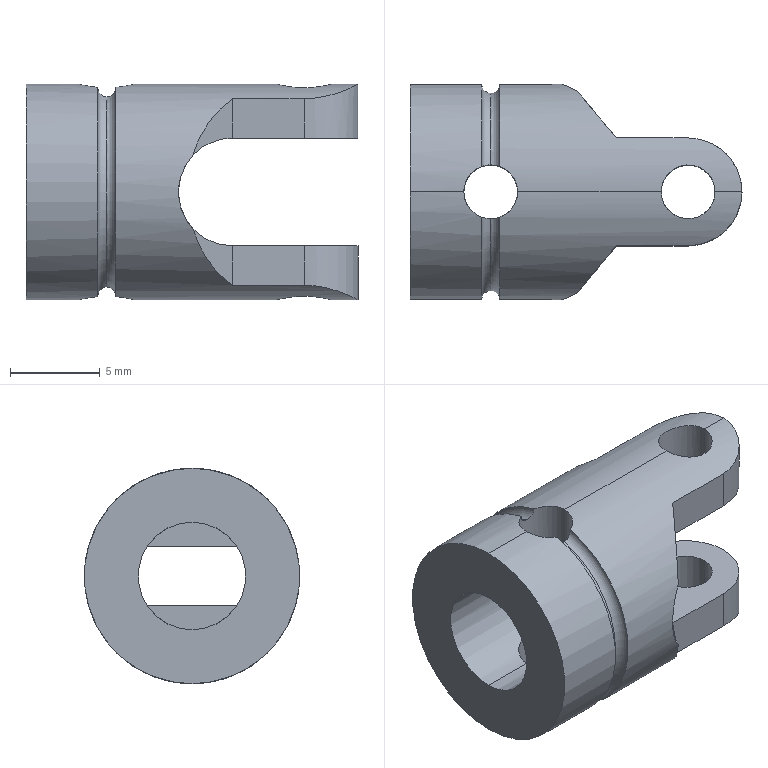Part | SolidWorks | features ICE 2, RefPoint 1, Revolution 1 | 1 solid | 36 faces | box 18.5 x 12 x 12 mm | volume 994.075 mm3 | cylinder 19 | plane 13 | torus 4 | commonest cylinder face diameters 3 x8 6 x7 12 x4